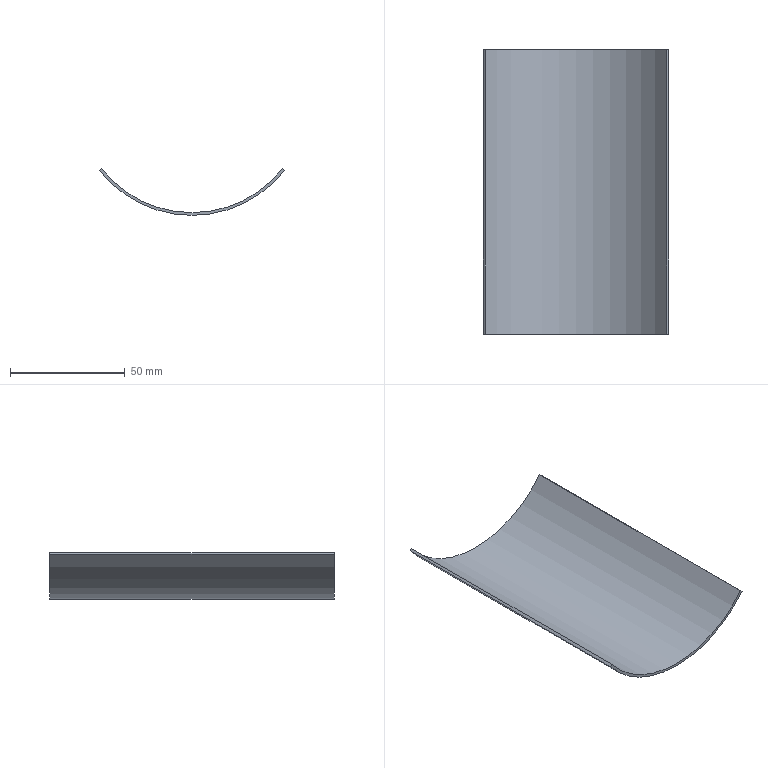Part | STEP file | JBJ-P-1003-06 | 1 solid | 6 faces | box 80.887 x 124 x 20.389 mm | volume 13687 mm3 | plane 4 | cylinder 2 | commonest cylinder face diameters 100.5 x1 102.9 x1
STEP:
#1=CARTESIAN_POINT('',(40.443,0.,-31.803));
#2=VERTEX_POINT('',#1);
#3=CARTESIAN_POINT('',(-40.443,0.,-31.803));
#4=VERTEX_POINT('',#3);
#5=CARTESIAN_POINT('',(0.,0.,0.));
#6=DIRECTION('',(0.,1.,0.));
#7=DIRECTION('',(1.,0.,0.));
#8=AXIS2_PLACEMENT_3D('',#5,#6,#7);
#9=CIRCLE('',#8,51.45);
#10=EDGE_CURVE('',#2,#4,#9,.T.);
#11=ORIENTED_EDGE('',*,*,#10,.T.);
#12=CARTESIAN_POINT('',(-40.443,124.,-31.803));
#13=VERTEX_POINT('',#12);
#14=CARTESIAN_POINT('',(-40.443,124.,-31.803));
#15=DIRECTION('',(0.,-1.,0.));
#16=VECTOR('',#15,1000.);
#17=LINE('',#14,#16);
#18=EDGE_CURVE('',#13,#4,#17,.T.);
#19=ORIENTED_EDGE('',*,*,#18,.F.);
#20=CARTESIAN_POINT('',(40.443,124.,-31.803));
#21=VERTEX_POINT('',#20);
#22=CARTESIAN_POINT('',(0.,124.,0.));
#23=DIRECTION('',(0.,1.,0.));
#24=DIRECTION('',(1.,0.,0.));
#25=AXIS2_PLACEMENT_3D('',#22,#23,#24);
#26=CIRCLE('',#25,51.45);
#27=EDGE_CURVE('',#21,#13,#26,.T.);
#28=ORIENTED_EDGE('',*,*,#27,.F.);
#29=CARTESIAN_POINT('',(40.443,124.,-31.803));
#30=DIRECTION('',(0.,-1.,0.));
#31=VECTOR('',#30,1000.);
#32=LINE('',#29,#31);
#33=EDGE_CURVE('',#21,#2,#32,.T.);
#34=ORIENTED_EDGE('',*,*,#33,.T.);
#35=EDGE_LOOP('',(#11,#19,#28,#34));
#36=FACE_OUTER_BOUND('',#35,.T.);
#37=CARTESIAN_POINT('',(0.,124.,0.));
#38=DIRECTION('',(0.,-1.,0.));
#39=DIRECTION('',(0.,0.,-1.));
#40=AXIS2_PLACEMENT_3D('',#37,#38,#39);
#41=CYLINDRICAL_SURFACE('',#40,51.45);
#42=ADVANCED_FACE('',(#36),#41,.T.);
#43=CARTESIAN_POINT('',(-39.5,0.,-31.061));
#44=VERTEX_POINT('',#43);
#45=CARTESIAN_POINT('',(-39.5,0.,-31.061));
#46=DIRECTION('',(-0.7861,0.,-0.6181));
#47=VECTOR('',#46,1000.);
#48=LINE('',#45,#47);
#49=EDGE_CURVE('',#44,#4,#48,.T.);
#50=ORIENTED_EDGE('',*,*,#49,.F.);
#51=CARTESIAN_POINT('',(-39.5,124.,-31.061));
#52=VERTEX_POINT('',#51);
#53=CARTESIAN_POINT('',(-39.5,124.,-31.061));
#54=DIRECTION('',(0.,-1.,0.));
#55=VECTOR('',#54,1000.);
#56=LINE('',#53,#55);
#57=EDGE_CURVE('',#52,#44,#56,.T.);
#58=ORIENTED_EDGE('',*,*,#57,.F.);
#59=CARTESIAN_POINT('',(-39.5,124.,-31.061));
#60=DIRECTION('',(-0.7861,0.,-0.6181));
#61=VECTOR('',#60,1000.);
#62=LINE('',#59,#61);
#63=EDGE_CURVE('',#52,#13,#62,.T.);
#64=ORIENTED_EDGE('',*,*,#63,.T.);
#65=ORIENTED_EDGE('',*,*,#18,.T.);
#66=EDGE_LOOP('',(#50,#58,#64,#65));
#67=FACE_OUTER_BOUND('',#66,.T.);
#68=CARTESIAN_POINT('',(-39.5,124.,-31.061));
#69=DIRECTION('',(-0.6181,0.,0.7861));
#70=DIRECTION('',(0.7861,0.,0.6181));
#71=AXIS2_PLACEMENT_3D('',#68,#69,#70);
#72=PLANE('',#71);
#73=ADVANCED_FACE('',(#67),#72,.T.);
#74=CARTESIAN_POINT('',(39.5,0.,-31.061));
#75=VERTEX_POINT('',#74);
#76=CARTESIAN_POINT('',(0.,0.,0.));
#77=DIRECTION('',(0.,1.,0.));
#78=DIRECTION('',(0.,0.,1.));
#79=AXIS2_PLACEMENT_3D('',#76,#77,#78);
#80=CIRCLE('',#79,50.25);
#81=EDGE_CURVE('',#75,#44,#80,.T.);
#82=ORIENTED_EDGE('',*,*,#81,.F.);
#83=CARTESIAN_POINT('',(39.5,124.,-31.061));
#84=VERTEX_POINT('',#83);
#85=CARTESIAN_POINT('',(39.5,124.,-31.061));
#86=DIRECTION('',(0.,-1.,0.));
#87=VECTOR('',#86,1000.);
#88=LINE('',#85,#87);
#89=EDGE_CURVE('',#84,#75,#88,.T.);
#90=ORIENTED_EDGE('',*,*,#89,.F.);
#91=CARTESIAN_POINT('',(0.,124.,0.));
#92=DIRECTION('',(0.,1.,0.));
#93=DIRECTION('',(0.,0.,1.));
#94=AXIS2_PLACEMENT_3D('',#91,#92,#93);
#95=CIRCLE('',#94,50.25);
#96=EDGE_CURVE('',#84,#52,#95,.T.);
#97=ORIENTED_EDGE('',*,*,#96,.T.);
#98=ORIENTED_EDGE('',*,*,#57,.T.);
#99=EDGE_LOOP('',(#82,#90,#97,#98));
#100=FACE_OUTER_BOUND('',#99,.T.);
#101=CARTESIAN_POINT('',(0.,124.,0.));
#102=DIRECTION('',(0.,-1.,0.));
#103=DIRECTION('',(0.,0.,-1.));
#104=AXIS2_PLACEMENT_3D('',#101,#102,#103);
#105=CYLINDRICAL_SURFACE('',#104,50.25);
#106=ADVANCED_FACE('',(#100),#105,.F.);
#107=CARTESIAN_POINT('',(40.443,0.,-31.803));
#108=DIRECTION('',(-0.7861,0.,0.6181));
#109=VECTOR('',#108,1000.);
#110=LINE('',#107,#109);
#111=EDGE_CURVE('',#2,#75,#110,.T.);
#112=ORIENTED_EDGE('',*,*,#111,.F.);
#113=ORIENTED_EDGE('',*,*,#33,.F.);
#114=CARTESIAN_POINT('',(40.443,124.,-31.803));
#115=DIRECTION('',(-0.7861,0.,0.6181));
#116=VECTOR('',#115,1000.);
#117=LINE('',#114,#116);
#118=EDGE_CURVE('',#21,#84,#117,.T.);
#119=ORIENTED_EDGE('',*,*,#118,.T.);
#120=ORIENTED_EDGE('',*,*,#89,.T.);
#121=EDGE_LOOP('',(#112,#113,#119,#120));
#122=FACE_OUTER_BOUND('',#121,.T.);
#123=CARTESIAN_POINT('',(40.443,124.,-31.803));
#124=DIRECTION('',(0.6181,0.,0.7861));
#125=DIRECTION('',(0.7861,0.,-0.6181));
#126=AXIS2_PLACEMENT_3D('',#123,#124,#125);
#127=PLANE('',#126);
#128=ADVANCED_FACE('',(#122),#127,.T.);
#129=ORIENTED_EDGE('',*,*,#27,.T.);
#130=ORIENTED_EDGE('',*,*,#63,.F.);
#131=ORIENTED_EDGE('',*,*,#96,.F.);
#132=ORIENTED_EDGE('',*,*,#118,.F.);
#133=EDGE_LOOP('',(#129,#130,#131,#132));
#134=FACE_OUTER_BOUND('',#133,.T.);
#135=CARTESIAN_POINT('',(0.,124.,0.));
#136=DIRECTION('',(0.,1.,0.));
#137=DIRECTION('',(1.,0.,0.));
#138=AXIS2_PLACEMENT_3D('',#135,#136,#137);
#139=PLANE('',#138);
#140=ADVANCED_FACE('',(#134),#139,.T.);
#141=ORIENTED_EDGE('',*,*,#10,.F.);
#142=ORIENTED_EDGE('',*,*,#111,.T.);
#143=ORIENTED_EDGE('',*,*,#81,.T.);
#144=ORIENTED_EDGE('',*,*,#49,.T.);
#145=EDGE_LOOP('',(#141,#142,#143,#144));
#146=FACE_OUTER_BOUND('',#145,.T.);
#147=CARTESIAN_POINT('',(0.,0.,0.));
#148=DIRECTION('',(0.,1.,0.));
#149=DIRECTION('',(1.,0.,0.));
#150=AXIS2_PLACEMENT_3D('',#147,#148,#149);
#151=PLANE('',#150);
#152=ADVANCED_FACE('',(#146),#151,.F.);
#153=CLOSED_SHELL('',(#42,#73,#106,#128,#140,#152));
#154=MANIFOLD_SOLID_BREP('',#153);
#155=CARTESIAN_POINT('',(0.,0.,0.));
#156=DIRECTION('',(0.,0.,1.));
#157=DIRECTION('',(1.,0.,0.));
#158=AXIS2_PLACEMENT_3D('',#155,#156,#157);
#159=(LENGTH_UNIT()NAMED_UNIT(*)SI_UNIT(.MILLI.,.METRE.));
#160=UNCERTAINTY_MEASURE_WITH_UNIT(LENGTH_MEASURE(0.00001),#159,'','');
#161=(NAMED_UNIT(*)PLANE_ANGLE_UNIT()SI_UNIT($,.RADIAN.));
#162=(NAMED_UNIT(*)SI_UNIT($,.STERADIAN.)SOLID_ANGLE_UNIT());
#163=(GEOMETRIC_REPRESENTATION_CONTEXT(3)GLOBAL_UNCERTAINTY_ASSIGNED_CONTEXT((#160))GLOBAL_UNIT_ASSIGNED_CONTEXT((#159,#161,#162))REPRESENTATION_CONTEXT('',''));
#164=ADVANCED_BREP_SHAPE_REPRESENTATION('',(#154,#158),#163);